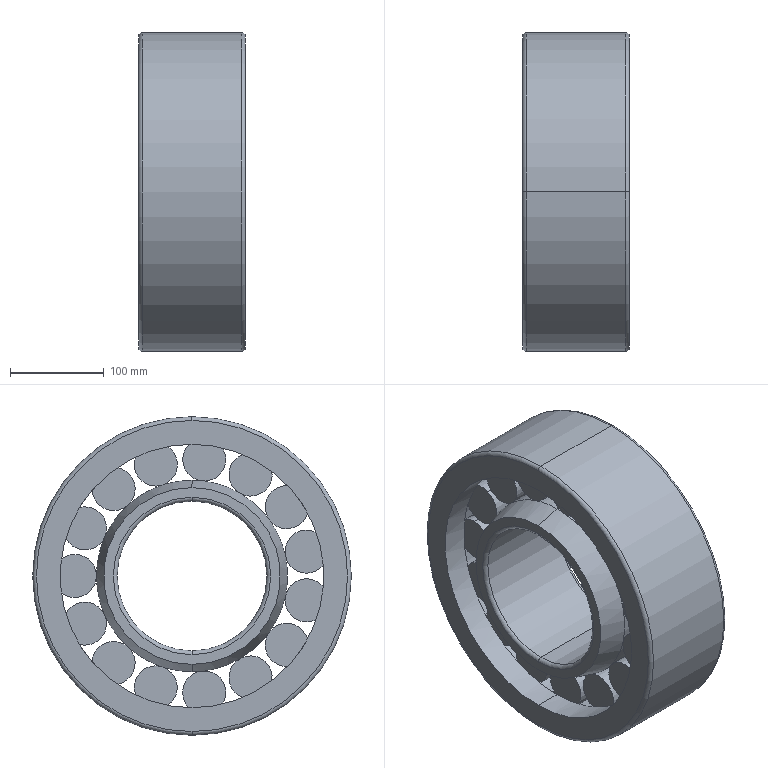Part | SolidWorks | features Revolution 3, Fillet 2, CirPattern 1 | 1 solid | 161 faces | box 114 x 340 x 340 mm | volume 5597424 mm3 | cylinder 85 | plane 64 | torus 8 | cone 4 | commonest cylinder face diameters 46.02 x45 204 x16 296 x16 281.2 x4 160 x2 340 x2